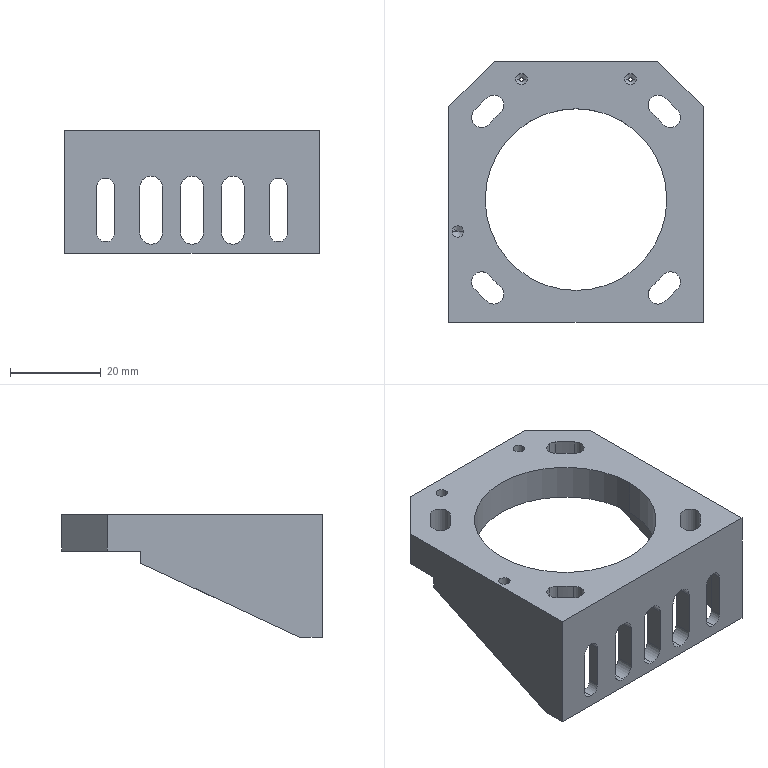NC program | NX | posted with a generic post | part box 56 x 57.4 x 27 mm
Lines 1 to 30 of 24340:
N10 G17 G21 G94 G90
(DRILLING , TOOL : ZXZ)
N12 T01 M6
N14 G54
N16 G17 G0 G90 X24.8 Y12. B0. C0. S3500 M3
N18 G43 Z30. H1
N20 G94 G81 G98 Z-1. F250. R3.
N22 Y-12.
N24 X-1.7 Y0.
N26 X-8.7 Y26.
N28 G80
N30 G0 X-8.7 Y26. Z30.
N32 M5
(DRILLING_COPY , TOOL : 2.5ZT)
N34 T12 M6
N36 G54
N38 G17 G0 G90 X24.8 Y-12. B0. C0. S2000 M3
N40 G43 Z30. H12
N42 G94 G83 G98 Z-8.251 F120. Q2. R3.
N44 Y12.
N46 X-8.7 Y26.
N48 G80
N50 G0 X-8.7 Y26. Z30.
N52 M5